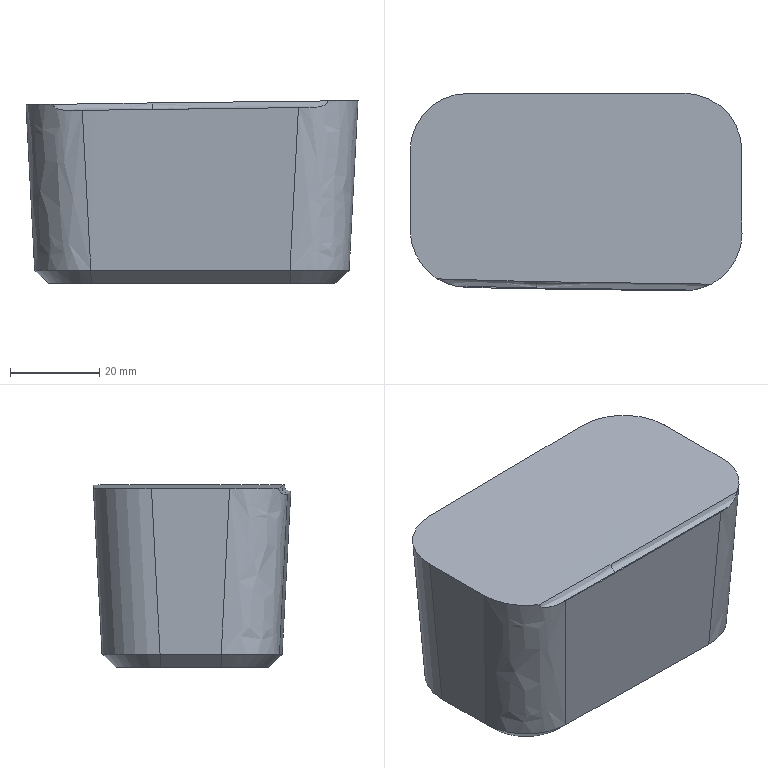Part | STEP file | solid 242 | 1 solid | 27 faces | box 74.238 x 44.192 x 40.9 mm | volume 109549 mm3 | spline 11 | plane 9 | cylinder 4 | cone 2 | other 1 | commonest cylinder face diameters 26 x2 10.2 x1 22 x1